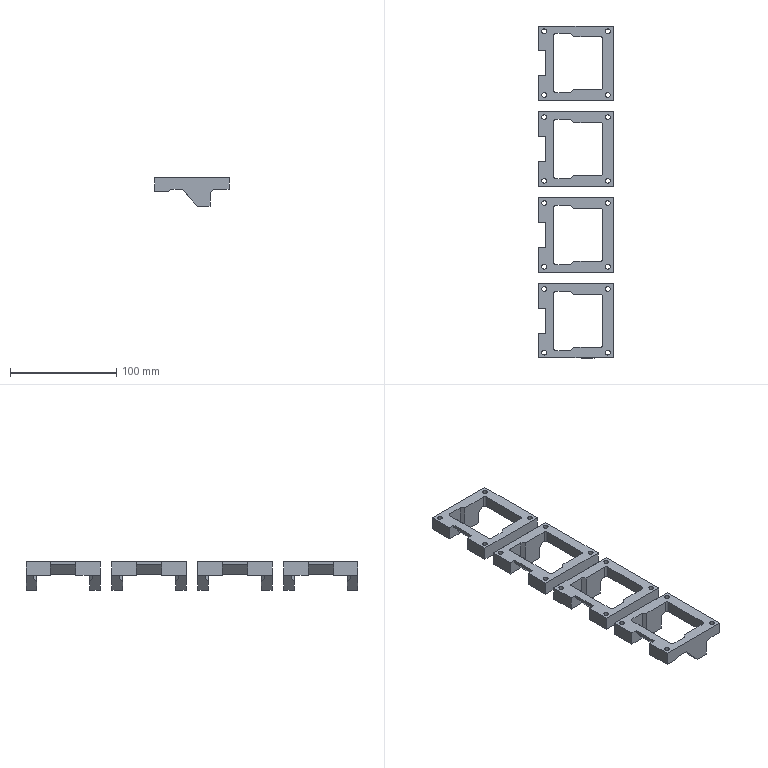NC program | NX | posted with a generic post | part box 70 x 313 x 26.9 mm
Lines 22850 to 23250 of 34421:
(CAVITY_MILL_COPY_1 , TOOL : D10JING)
N45692 T11 M6
N45694 G54
N45696 G17 G0 G90 X-139.691 Y3.622 S9500 M3
N45698 G43 Z30. H11
N45700 Z-12.45
N45702 G94 G1 Z-13.45 F1000.
N45704 X-141. Y2.866
N45706 G3 X-141.5 Y2. R1.
N45708 G1 Y-20. F1200.
N45710 X-101.5
N45712 Y2.
N45714 G2 X-100.036 Y5.536 R5.
N45716 G1 X-98.5 Y7.071
N45718 Y16.
N45720 X-144.5
N45722 Y7.071
N45724 X-142.964 Y5.536
N45726 G2 X-141.5 Y2. R5.
N45728 G3 X-141. Y1.134 R1.
N45730 G1 X-139.5 Y0.268
N45732 Z-12.45
N45734 G0 Z30.
N45736 X-139.691 Y3.622
N45738 Z-25.9
N45740 G1 Z-26.9 F1000.
N45742 X-141. Y2.866
N45744 G3 X-141.5 Y2. R1.
N45746 G1 Y-20. F1200.
N45748 X-101.5
N45750 Y2.
N45752 G2 X-100.036 Y5.536 R5.
N45754 G1 X-98.5 Y7.071
N45756 Y16.
N45758 X-144.5
N45760 Y7.071
N45762 X-142.964 Y5.536
N45764 G2 X-141.5 Y2. R5.
N45766 G3 X-141. Y1.134 R1.
N45768 G1 X-139.5 Y0.268
N45770 Z-25.9
N45772 G0 Z30.
N45774 X-58.691 Y3.622
N45776 Z-12.45
N45778 G1 Z-13.45 F1000.
N45780 X-60. Y2.866
N45782 G3 X-60.5 Y2. R1.
N45784 G1 Y-20. F1200.
N45786 X-20.5
N45788 Y2.
N45790 G2 X-19.036 Y5.536 R5.
N45792 G1 X-17.5 Y7.071
N45794 Y16.
N45796 X-63.5
N45798 Y7.071
N45800 X-61.964 Y5.536
N45802 G2 X-60.5 Y2. R5.
N45804 G3 X-60. Y1.134 R1.
N45806 G1 X-58.5 Y0.268
N45808 Z-12.45
N45810 G0 Z30.
N45812 X-58.691 Y3.622
N45814 Z-25.9
N45816 G1 Z-26.9 F1000.
N45818 X-60. Y2.866
N45820 G3 X-60.5 Y2. R1.
N45822 G1 Y-20. F1200.
N45824 X-20.5
N45826 Y2.
N45828 G2 X-19.036 Y5.536 R5.
N45830 G1 X-17.5 Y7.071
N45832 Y16.
N45834 X-63.5
N45836 Y7.071
N45838 X-61.964 Y5.536
N45840 G2 X-60.5 Y2. R5.
N45842 G3 X-60. Y1.134 R1.
N45844 G1 X-58.5 Y0.268
N45846 Z-25.9
N45848 G0 Z30.
N45850 X-84.878 Y-41.809
N45852 Z-12.45
N45854 G1 Z-13.45 F1000.
N45856 X-85.634 Y-40.5
N45858 G3 X-86.5 Y-40. R1.
N45860 G1 X-156.5 F1200.
N45862 G2 X-161.5 Y-35. R5.
N45864 G1 Y35.
N45866 G2 X-156.5 Y40. R5.
N45868 G1 X-133.5
N45870 G2 X-128.5 Y35. R5.
N45872 G1 Y34.204
N45874 X-114.5
N45876 Y35.
N45878 G2 X-109.5 Y40. R5.
N45880 G1 X-86.5
N45882 G2 X-81.5 Y35. R5.
N45884 G1 Y-35.
N45886 G2 X-86.5 Y-40. R5.
N45888 G3 X-87.366 Y-40.5 R1.
N45890 G1 X-88.232 Y-42.
N45892 Z-12.45
N45894 G0 Z30.
N45896 X-38.768
N45898 Z-12.45
N45900 G1 Z-13.45 F1000.
N45902 X-39.634 Y-40.5
N45904 G3 X-40.5 Y-40. R1.
N45906 G1 X-75.5 F1200.
N45908 G2 X-80.5 Y-35. R5.
N45910 G1 Y35.
N45912 G2 X-75.5 Y40. R5.
N45914 G1 X-52.5
N45916 G2 X-47.5 Y35. R5.
N45918 G1 Y34.204
N45920 X-33.5
N45922 Y35.
N45924 G2 X-28.5 Y40. R5.
N45926 G1 X-5.5
N45928 G2 X-0.5 Y35. R5.
N45930 G1 Y-35.
N45932 G2 X-5.5 Y-40. R5.
N45934 G1 X-40.5
N45936 G3 X-41.366 Y-40.5 R1.
N45938 G1 X-42.232 Y-42.
N45940 Z-12.45
N45942 G0 Z30.
N45944 X42.232
N45946 Z-12.45
N45948 G1 Z-13.45 F1000.
N45950 X41.366 Y-40.5
N45952 G3 X40.5 Y-40. R1.
N45954 G1 X5.5 F1200.
N45956 G2 X0.5 Y-35. R5.
N45958 G1 Y35.
N45960 G2 X5.5 Y40. R5.
N45962 G1 X28.5
N45964 G2 X33.5 Y35. R5.
N45966 G1 Y34.204
N45968 X47.5
N45970 Y35.
N45972 G2 X52.5 Y40. R5.
N45974 G1 X75.5
N45976 G2 X80.5 Y35. R5.
N45978 G1 Y-35.
N45980 G2 X75.5 Y-40. R5.
N45982 G1 X40.5
N45984 G3 X39.634 Y-40.5 R1.
N45986 G1 X38.768 Y-42.
N45988 Z-12.45
N45990 G0 Z30.
N45992 X123.232
N45994 Z-12.45
N45996 G1 Z-13.45 F1000.
N45998 X122.366 Y-40.5
N46000 G3 X121.5 Y-40. R1.
N46002 G1 X86.5 F1200.
N46004 G2 X81.5 Y-35. R5.
N46006 G1 Y35.
N46008 G2 X86.5 Y40. R5.
N46010 G1 X109.5
N46012 G2 X114.5 Y35. R5.
N46014 G1 Y34.204
N46016 X128.5
N46018 Y35.
N46020 G2 X133.5 Y40. R5.
N46022 G1 X156.5
N46024 G2 X161.5 Y35. R5.
N46026 G1 Y-35.
N46028 G2 X156.5 Y-40. R5.
N46030 G1 X121.5
N46032 G3 X120.634 Y-40.5 R1.
N46034 G1 X119.768 Y-42.
N46036 Z-12.45
N46038 G0 Z30.
N46040 X158.122 Y-41.809
N46042 Z-25.9
N46044 G1 Z-26.9 F1000.
N46046 X157.366 Y-40.5
N46048 G3 X156.5 Y-40. R1.
N46050 G1 X86.5 F1200.
N46052 G2 X81.5 Y-35. R5.
N46054 G1 Y35.
N46056 G2 X86.5 Y40. R5.
N46058 G1 X109.5
N46060 G2 X114.5 Y35. R5.
N46062 G1 Y34.204
N46064 X128.5
N46066 Y35.
N46068 G2 X133.5 Y40. R5.
N46070 G1 X156.5
N46072 G2 X161.5 Y35. R5.
N46074 G1 Y-35.
N46076 G2 X156.5 Y-40. R5.
N46078 G3 X155.634 Y-40.5 R1.
N46080 G1 X154.768 Y-42.
N46082 Z-25.9
N46084 G0 Z-10.45
N46086 X42.232
N46088 Z-25.9
N46090 G1 Z-26.9 F1000.
N46092 X41.366 Y-40.5
N46094 G3 X40.5 Y-40. R1.
N46096 G1 X5.5 F1200.
N46098 G2 X0.5 Y-35. R5.
N46100 G1 Y35.
N46102 G2 X5.5 Y40. R5.
N46104 G1 X28.5
N46106 G2 X33.5 Y35. R5.
N46108 G1 Y34.204
N46110 X47.5
N46112 Y35.
N46114 G2 X52.5 Y40. R5.
N46116 G1 X75.5
N46118 G2 X80.5 Y35. R5.
N46120 G1 Y-35.
N46122 G2 X75.5 Y-40. R5.
N46124 G1 X40.5
N46126 G3 X39.634 Y-40.5 R1.
N46128 G1 X38.768 Y-42.
N46130 Z-25.9
N46132 G0 Z-10.45
N46134 X-38.768
N46136 Z-25.9
N46138 G1 Z-26.9 F1000.
N46140 X-39.634 Y-40.5
N46142 G3 X-40.5 Y-40. R1.
N46144 G1 X-75.5 F1200.
N46146 G2 X-80.5 Y-35. R5.
N46148 G1 Y35.
N46150 G2 X-75.5 Y40. R5.
N46152 G1 X-52.5
N46154 G2 X-47.5 Y35. R5.
N46156 G1 Y34.204
N46158 X-33.5
N46160 Y35.
N46162 G2 X-28.5 Y40. R5.
N46164 G1 X-5.5
N46166 G2 X-0.5 Y35. R5.
N46168 G1 Y-35.
N46170 G2 X-5.5 Y-40. R5.
N46172 G1 X-40.5
N46174 G3 X-41.366 Y-40.5 R1.
N46176 G1 X-42.232 Y-42.
N46178 Z-25.9
N46180 G0 Z-10.45
N46182 X-119.768
N46184 Z-25.9
N46186 G1 Z-26.9 F1000.
N46188 X-120.634 Y-40.5
N46190 G3 X-121.5 Y-40. R1.
N46192 G1 X-156.5 F1200.
N46194 G2 X-161.5 Y-35. R5.
N46196 G1 Y35.
N46198 G2 X-156.5 Y40. R5.
N46200 G1 X-133.5
N46202 G2 X-128.5 Y35. R5.
N46204 G1 Y34.204
N46206 X-114.5
N46208 Y35.
N46210 G2 X-109.5 Y40. R5.
N46212 G1 X-86.5
N46214 G2 X-81.5 Y35. R5.
N46216 G1 Y-35.
N46218 G2 X-86.5 Y-40. R5.
N46220 G1 X-121.5
N46222 G3 X-122.366 Y-40.5 R1.
N46224 G1 X-123.232 Y-42.
N46226 Z-25.9
N46228 G0 Z30.
N46230 X22.309 Y3.622
N46232 Z-12.45
N46234 G1 Z-13.45 F1000.
N46236 X21. Y2.866
N46238 G3 X20.5 Y2. R1.
N46240 G1 Y-20. F1200.
N46242 X60.5
N46244 Y2.
N46246 G2 X61.964 Y5.536 R5.
N46248 G1 X63.5 Y7.071
N46250 Y16.
N46252 X17.5
N46254 Y7.071
N46256 X19.036 Y5.536
N46258 G2 X20.5 Y2. R5.
N46260 G3 X21. Y1.134 R1.
N46262 G1 X22.5 Y0.268
N46264 Z-12.45
N46266 G0 Z30.
N46268 X22.309 Y3.622
N46270 Z-25.9
N46272 G1 Z-26.9 F1000.
N46274 X21. Y2.866
N46276 G3 X20.5 Y2. R1.
N46278 G1 Y-20. F1200.
N46280 X60.5
N46282 Y2.
N46284 G2 X61.964 Y5.536 R5.
N46286 G1 X63.5 Y7.071
N46288 Y16.
N46290 X17.5
N46292 Y7.071
N46294 X19.036 Y5.536
N46296 G2 X20.5 Y2. R5.
N46298 G3 X21. Y1.134 R1.
N46300 G1 X22.5 Y0.268
N46302 Z-25.9
N46304 G0 Z30.
N46306 X103.309 Y3.622
N46308 Z-12.45
N46310 G1 Z-13.45 F1000.
N46312 X102. Y2.866
N46314 G3 X101.5 Y2. R1.
N46316 G1 Y-20. F1200.
N46318 X141.5
N46320 Y2.
N46322 G2 X142.964 Y5.536 R5.
N46324 G1 X144.5 Y7.071
N46326 Y16.
N46328 X98.5
N46330 Y7.071
N46332 X100.036 Y5.536
N46334 G2 X101.5 Y2. R5.
N46336 G3 X102. Y1.134 R1.
N46338 G1 X103.5 Y0.268
N46340 Z-12.45
N46342 G0 Z30.
N46344 X103.309 Y3.622
N46346 Z-25.9
N46348 G1 Z-26.9 F1000.
N46350 X102. Y2.866
N46352 G3 X101.5 Y2. R1.
N46354 G1 Y-20. F1200.
N46356 X141.5
N46358 Y2.
N46360 G2 X142.964 Y5.536 R5.
N46362 G1 X144.5 Y7.071
N46364 Y16.
N46366 X98.5
N46368 Y7.071
N46370 X100.036 Y5.536
N46372 G2 X101.5 Y2. R5.
N46374 G3 X102. Y1.134 R1.
N46376 G1 X103.5 Y0.268
N46378 Z-25.9
N46380 G0 Z30.
N46382 M5
(DRILLING , TOOL : D6A45)
N46384 T07 M6
N46386 G54
N46388 G17 G0 G90 X-151.5 Y-30. S5000 M3
N46390 G43 Z30. H7
N46392 G94 G81 G98 Z-17. F250. R-13.
N46394 X-91.5
N46396 X-70.5
N46398 X-10.5
N46400 X10.5
N46402 X70.5
N46404 X91.5
N46406 X151.5
N46408 Y30.
N46410 X91.5
N46412 X70.5
N46414 X10.5
N46416 X-10.5
N46418 X-70.5
N46420 X-91.5
N46422 X-151.5
N46424 G80
N46426 G0 X-151.5 Y30. Z30.
N46428 M5
(DRILLING_COPY , TOOL : 4.5ZT)
N46430 T14 M6
N46432 G54
N46434 G17 G0 G90 X-151.5 Y-30. S2000 M3
N46436 G43 Z30. H14
N46438 G94 G83 G98 Z-28.352 F200. Q2. R-13.
N46440 X-91.5
N46442 X-70.5
N46444 X-10.5
N46446 X10.5
N46448 X70.5
N46450 X91.5
N46452 X151.5
N46454 Y30.
N46456 X91.5
N46458 X70.5
N46460 X10.5
N46462 X-10.5
N46464 X-70.5
N46466 X-91.5
N46468 X-151.5
N46470 G80
N46472 G0 X-151.5 Y30. Z30.
N46474 M5